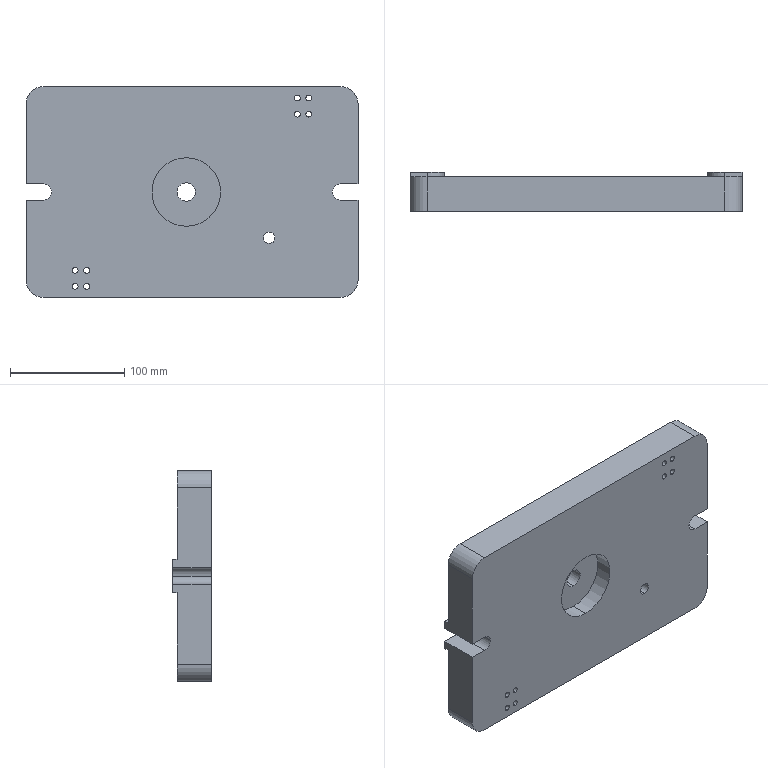Part | SolidWorks | features ICE 7, Fillet 2, Extrusion 1, HoleWzd 1 | 1 solid | 53 faces | box 290 x 34 x 184 mm | volume 1528919 mm3 | cylinder 34 | plane 19 | commonest cylinder face diameters 5 x16 30 x8 15 x4 10 x2 16 x2 60 x2